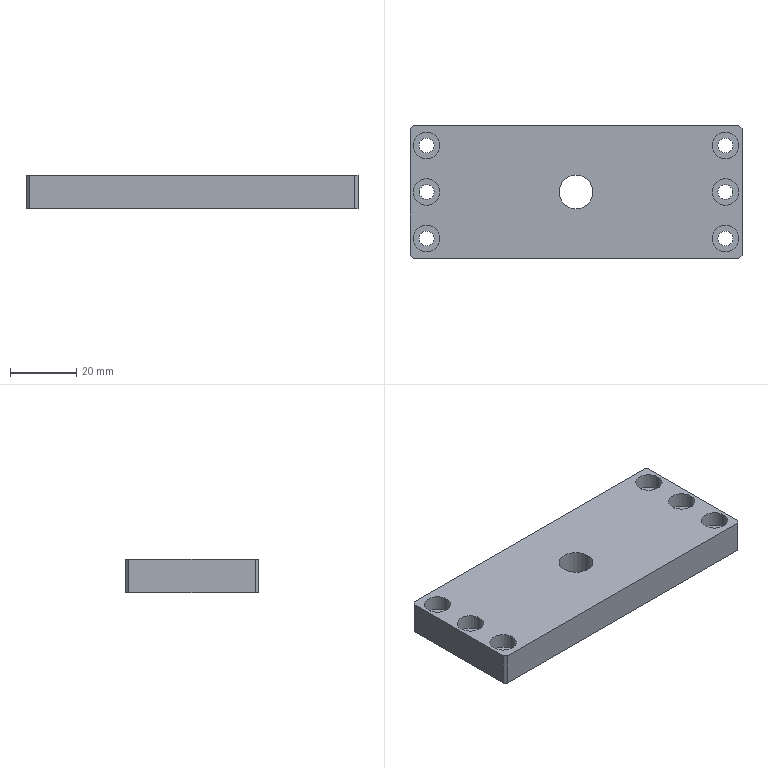Part | STEP file | MYT-A01-P12 | 1 solid | 42 faces | box 100 x 40 x 10 mm | volume 37260 mm3 | cylinder 26 | plane 16 | commonest cylinder face diameters 4.5 x12 8 x12 10.2 x2
STEP:
#1=CARTESIAN_POINT('',(-5.1,0.,0.));
#2=VERTEX_POINT('',#1);
#3=CARTESIAN_POINT('',(5.1,0.,0.));
#4=VERTEX_POINT('',#3);
#5=CARTESIAN_POINT('',(0.,0.,0.));
#6=DIRECTION('',(0.,0.,1.));
#7=DIRECTION('',(1.,0.,0.));
#8=AXIS2_PLACEMENT_3D('',#5,#6,#7);
#9=CIRCLE('',#8,5.1);
#10=EDGE_CURVE('',#2,#4,#9,.T.);
#11=ORIENTED_EDGE('',*,*,#10,.F.);
#12=CARTESIAN_POINT('',(-5.1,0.,10.));
#13=VERTEX_POINT('',#12);
#14=CARTESIAN_POINT('',(-5.1,0.,10.));
#15=DIRECTION('',(0.,0.,1.));
#16=VECTOR('',#15,1000.);
#17=LINE('',#14,#16);
#18=EDGE_CURVE('',#2,#13,#17,.T.);
#19=ORIENTED_EDGE('',*,*,#18,.T.);
#20=CARTESIAN_POINT('',(5.1,0.,10.));
#21=VERTEX_POINT('',#20);
#22=CARTESIAN_POINT('',(0.,0.,10.));
#23=DIRECTION('',(0.,0.,1.));
#24=DIRECTION('',(1.,0.,0.));
#25=AXIS2_PLACEMENT_3D('',#22,#23,#24);
#26=CIRCLE('',#25,5.1);
#27=EDGE_CURVE('',#13,#21,#26,.T.);
#28=ORIENTED_EDGE('',*,*,#27,.T.);
#29=CARTESIAN_POINT('',(5.1,0.,10.));
#30=DIRECTION('',(0.,0.,1.));
#31=VECTOR('',#30,1000.);
#32=LINE('',#29,#31);
#33=EDGE_CURVE('',#4,#21,#32,.T.);
#34=ORIENTED_EDGE('',*,*,#33,.F.);
#35=EDGE_LOOP('',(#11,#19,#28,#34));
#36=FACE_OUTER_BOUND('',#35,.T.);
#37=CARTESIAN_POINT('',(0.,0.,10.));
#38=DIRECTION('',(0.,0.,1.));
#39=DIRECTION('',(1.,0.,0.));
#40=AXIS2_PLACEMENT_3D('',#37,#38,#39);
#41=CYLINDRICAL_SURFACE('',#40,5.1);
#42=ADVANCED_FACE('',(#36),#41,.F.);
#43=CARTESIAN_POINT('',(-49.,14.,5.4));
#44=VERTEX_POINT('',#43);
#45=CARTESIAN_POINT('',(-41.,14.,5.4));
#46=VERTEX_POINT('',#45);
#47=CARTESIAN_POINT('',(-45.,14.,5.4));
#48=DIRECTION('',(0.,0.,1.));
#49=DIRECTION('',(1.,0.,0.));
#50=AXIS2_PLACEMENT_3D('',#47,#48,#49);
#51=CIRCLE('',#50,4.);
#52=EDGE_CURVE('',#44,#46,#51,.T.);
#53=ORIENTED_EDGE('',*,*,#52,.F.);
#54=CARTESIAN_POINT('',(-49.,14.,10.));
#55=VERTEX_POINT('',#54);
#56=CARTESIAN_POINT('',(-49.,14.,10.));
#57=DIRECTION('',(0.,0.,1.));
#58=VECTOR('',#57,1000.);
#59=LINE('',#56,#58);
#60=EDGE_CURVE('',#44,#55,#59,.T.);
#61=ORIENTED_EDGE('',*,*,#60,.T.);
#62=CARTESIAN_POINT('',(-41.,14.,10.));
#63=VERTEX_POINT('',#62);
#64=CARTESIAN_POINT('',(-45.,14.,10.));
#65=DIRECTION('',(0.,0.,1.));
#66=DIRECTION('',(1.,0.,0.));
#67=AXIS2_PLACEMENT_3D('',#64,#65,#66);
#68=CIRCLE('',#67,4.);
#69=EDGE_CURVE('',#55,#63,#68,.T.);
#70=ORIENTED_EDGE('',*,*,#69,.T.);
#71=CARTESIAN_POINT('',(-41.,14.,10.));
#72=DIRECTION('',(0.,0.,1.));
#73=VECTOR('',#72,1000.);
#74=LINE('',#71,#73);
#75=EDGE_CURVE('',#46,#63,#74,.T.);
#76=ORIENTED_EDGE('',*,*,#75,.F.);
#77=EDGE_LOOP('',(#53,#61,#70,#76));
#78=FACE_OUTER_BOUND('',#77,.T.);
#79=CARTESIAN_POINT('',(-45.,14.,10.));
#80=DIRECTION('',(0.,0.,1.));
#81=DIRECTION('',(1.,0.,0.));
#82=AXIS2_PLACEMENT_3D('',#79,#80,#81);
#83=CYLINDRICAL_SURFACE('',#82,4.);
#84=ADVANCED_FACE('',(#78),#83,.F.);
#85=CARTESIAN_POINT('',(-42.75,14.,0.));
#86=VERTEX_POINT('',#85);
#87=CARTESIAN_POINT('',(-47.25,14.,0.));
#88=VERTEX_POINT('',#87);
#89=CARTESIAN_POINT('',(-45.,14.,0.));
#90=DIRECTION('',(0.,0.,-1.));
#91=DIRECTION('',(-1.,0.,0.));
#92=AXIS2_PLACEMENT_3D('',#89,#90,#91);
#93=CIRCLE('',#92,2.25);
#94=EDGE_CURVE('',#86,#88,#93,.T.);
#95=ORIENTED_EDGE('',*,*,#94,.T.);
#96=CARTESIAN_POINT('',(-47.25,14.,5.4));
#97=VERTEX_POINT('',#96);
#98=CARTESIAN_POINT('',(-47.25,14.,10.));
#99=DIRECTION('',(0.,0.,1.));
#100=VECTOR('',#99,1000.);
#101=LINE('',#98,#100);
#102=EDGE_CURVE('',#88,#97,#101,.T.);
#103=ORIENTED_EDGE('',*,*,#102,.T.);
#104=CARTESIAN_POINT('',(-42.75,14.,5.4));
#105=VERTEX_POINT('',#104);
#106=CARTESIAN_POINT('',(-45.,14.,5.4));
#107=DIRECTION('',(0.,0.,1.));
#108=DIRECTION('',(1.,0.,0.));
#109=AXIS2_PLACEMENT_3D('',#106,#107,#108);
#110=CIRCLE('',#109,2.25);
#111=EDGE_CURVE('',#97,#105,#110,.T.);
#112=ORIENTED_EDGE('',*,*,#111,.T.);
#113=CARTESIAN_POINT('',(-42.75,14.,10.));
#114=DIRECTION('',(0.,0.,1.));
#115=VECTOR('',#114,1000.);
#116=LINE('',#113,#115);
#117=EDGE_CURVE('',#86,#105,#116,.T.);
#118=ORIENTED_EDGE('',*,*,#117,.F.);
#119=EDGE_LOOP('',(#95,#103,#112,#118));
#120=FACE_OUTER_BOUND('',#119,.T.);
#121=CARTESIAN_POINT('',(-45.,14.,10.));
#122=DIRECTION('',(0.,0.,1.));
#123=DIRECTION('',(1.,0.,0.));
#124=AXIS2_PLACEMENT_3D('',#121,#122,#123);
#125=CYLINDRICAL_SURFACE('',#124,2.25);
#126=ADVANCED_FACE('',(#120),#125,.F.);
#127=CARTESIAN_POINT('',(-49.,0.,5.4));
#128=VERTEX_POINT('',#127);
#129=CARTESIAN_POINT('',(-41.,0.,5.4));
#130=VERTEX_POINT('',#129);
#131=CARTESIAN_POINT('',(-45.,0.,5.4));
#132=DIRECTION('',(0.,0.,1.));
#133=DIRECTION('',(1.,0.,0.));
#134=AXIS2_PLACEMENT_3D('',#131,#132,#133);
#135=CIRCLE('',#134,4.);
#136=EDGE_CURVE('',#128,#130,#135,.T.);
#137=ORIENTED_EDGE('',*,*,#136,.F.);
#138=CARTESIAN_POINT('',(-49.,0.,10.));
#139=VERTEX_POINT('',#138);
#140=CARTESIAN_POINT('',(-49.,0.,10.));
#141=DIRECTION('',(0.,0.,1.));
#142=VECTOR('',#141,1000.);
#143=LINE('',#140,#142);
#144=EDGE_CURVE('',#128,#139,#143,.T.);
#145=ORIENTED_EDGE('',*,*,#144,.T.);
#146=CARTESIAN_POINT('',(-41.,0.,10.));
#147=VERTEX_POINT('',#146);
#148=CARTESIAN_POINT('',(-45.,0.,10.));
#149=DIRECTION('',(0.,0.,1.));
#150=DIRECTION('',(1.,0.,0.));
#151=AXIS2_PLACEMENT_3D('',#148,#149,#150);
#152=CIRCLE('',#151,4.);
#153=EDGE_CURVE('',#139,#147,#152,.T.);
#154=ORIENTED_EDGE('',*,*,#153,.T.);
#155=CARTESIAN_POINT('',(-41.,0.,10.));
#156=DIRECTION('',(0.,0.,1.));
#157=VECTOR('',#156,1000.);
#158=LINE('',#155,#157);
#159=EDGE_CURVE('',#130,#147,#158,.T.);
#160=ORIENTED_EDGE('',*,*,#159,.F.);
#161=EDGE_LOOP('',(#137,#145,#154,#160));
#162=FACE_OUTER_BOUND('',#161,.T.);
#163=CARTESIAN_POINT('',(-45.,0.,10.));
#164=DIRECTION('',(0.,0.,1.));
#165=DIRECTION('',(1.,0.,0.));
#166=AXIS2_PLACEMENT_3D('',#163,#164,#165);
#167=CYLINDRICAL_SURFACE('',#166,4.);
#168=ADVANCED_FACE('',(#162),#167,.F.);
#169=CARTESIAN_POINT('',(-42.75,0.,0.));
#170=VERTEX_POINT('',#169);
#171=CARTESIAN_POINT('',(-47.25,0.,0.));
#172=VERTEX_POINT('',#171);
#173=CARTESIAN_POINT('',(-45.,0.,0.));
#174=DIRECTION('',(0.,0.,-1.));
#175=DIRECTION('',(-1.,0.,0.));
#176=AXIS2_PLACEMENT_3D('',#173,#174,#175);
#177=CIRCLE('',#176,2.25);
#178=EDGE_CURVE('',#170,#172,#177,.T.);
#179=ORIENTED_EDGE('',*,*,#178,.T.);
#180=CARTESIAN_POINT('',(-47.25,0.,5.4));
#181=VERTEX_POINT('',#180);
#182=CARTESIAN_POINT('',(-47.25,0.,10.));
#183=DIRECTION('',(0.,0.,1.));
#184=VECTOR('',#183,1000.);
#185=LINE('',#182,#184);
#186=EDGE_CURVE('',#172,#181,#185,.T.);
#187=ORIENTED_EDGE('',*,*,#186,.T.);
#188=CARTESIAN_POINT('',(-42.75,0.,5.4));
#189=VERTEX_POINT('',#188);
#190=CARTESIAN_POINT('',(-45.,0.,5.4));
#191=DIRECTION('',(0.,0.,1.));
#192=DIRECTION('',(1.,0.,0.));
#193=AXIS2_PLACEMENT_3D('',#190,#191,#192);
#194=CIRCLE('',#193,2.25);
#195=EDGE_CURVE('',#181,#189,#194,.T.);
#196=ORIENTED_EDGE('',*,*,#195,.T.);
#197=CARTESIAN_POINT('',(-42.75,0.,10.));
#198=DIRECTION('',(0.,0.,1.));
#199=VECTOR('',#198,1000.);
#200=LINE('',#197,#199);
#201=EDGE_CURVE('',#170,#189,#200,.T.);
#202=ORIENTED_EDGE('',*,*,#201,.F.);
#203=EDGE_LOOP('',(#179,#187,#196,#202));
#204=FACE_OUTER_BOUND('',#203,.T.);
#205=CARTESIAN_POINT('',(-45.,0.,10.));
#206=DIRECTION('',(0.,0.,1.));
#207=DIRECTION('',(1.,0.,0.));
#208=AXIS2_PLACEMENT_3D('',#205,#206,#207);
#209=CYLINDRICAL_SURFACE('',#208,2.25);
#210=ADVANCED_FACE('',(#204),#209,.F.);
#211=CARTESIAN_POINT('',(-49.,-14.,5.4));
#212=VERTEX_POINT('',#211);
#213=CARTESIAN_POINT('',(-41.,-14.,5.4));
#214=VERTEX_POINT('',#213);
#215=CARTESIAN_POINT('',(-45.,-14.,5.4));
#216=DIRECTION('',(0.,0.,1.));
#217=DIRECTION('',(1.,0.,0.));
#218=AXIS2_PLACEMENT_3D('',#215,#216,#217);
#219=CIRCLE('',#218,4.);
#220=EDGE_CURVE('',#212,#214,#219,.T.);
#221=ORIENTED_EDGE('',*,*,#220,.F.);
#222=CARTESIAN_POINT('',(-49.,-14.,10.));
#223=VERTEX_POINT('',#222);
#224=CARTESIAN_POINT('',(-49.,-14.,10.));
#225=DIRECTION('',(0.,0.,1.));
#226=VECTOR('',#225,1000.);
#227=LINE('',#224,#226);
#228=EDGE_CURVE('',#212,#223,#227,.T.);
#229=ORIENTED_EDGE('',*,*,#228,.T.);
#230=CARTESIAN_POINT('',(-41.,-14.,10.));
#231=VERTEX_POINT('',#230);
#232=CARTESIAN_POINT('',(-45.,-14.,10.));
#233=DIRECTION('',(0.,0.,1.));
#234=DIRECTION('',(1.,0.,0.));
#235=AXIS2_PLACEMENT_3D('',#232,#233,#234);
#236=CIRCLE('',#235,4.);
#237=EDGE_CURVE('',#223,#231,#236,.T.);
#238=ORIENTED_EDGE('',*,*,#237,.T.);
#239=CARTESIAN_POINT('',(-41.,-14.,10.));
#240=DIRECTION('',(0.,0.,1.));
#241=VECTOR('',#240,1000.);
#242=LINE('',#239,#241);
#243=EDGE_CURVE('',#214,#231,#242,.T.);
#244=ORIENTED_EDGE('',*,*,#243,.F.);
#245=EDGE_LOOP('',(#221,#229,#238,#244));
#246=FACE_OUTER_BOUND('',#245,.T.);
#247=CARTESIAN_POINT('',(-45.,-14.,10.));
#248=DIRECTION('',(0.,0.,1.));
#249=DIRECTION('',(1.,0.,0.));
#250=AXIS2_PLACEMENT_3D('',#247,#248,#249);
#251=CYLINDRICAL_SURFACE('',#250,4.);
#252=ADVANCED_FACE('',(#246),#251,.F.);
#253=CARTESIAN_POINT('',(-42.75,-14.,0.));
#254=VERTEX_POINT('',#253);
#255=CARTESIAN_POINT('',(-47.25,-14.,0.));
#256=VERTEX_POINT('',#255);
#257=CARTESIAN_POINT('',(-45.,-14.,0.));
#258=DIRECTION('',(0.,0.,-1.));
#259=DIRECTION('',(-1.,0.,0.));
#260=AXIS2_PLACEMENT_3D('',#257,#258,#259);
#261=CIRCLE('',#260,2.25);
#262=EDGE_CURVE('',#254,#256,#261,.T.);
#263=ORIENTED_EDGE('',*,*,#262,.T.);
#264=CARTESIAN_POINT('',(-47.25,-14.,5.4));
#265=VERTEX_POINT('',#264);
#266=CARTESIAN_POINT('',(-47.25,-14.,10.));
#267=DIRECTION('',(0.,0.,1.));
#268=VECTOR('',#267,1000.);
#269=LINE('',#266,#268);
#270=EDGE_CURVE('',#256,#265,#269,.T.);
#271=ORIENTED_EDGE('',*,*,#270,.T.);
#272=CARTESIAN_POINT('',(-42.75,-14.,5.4));
#273=VERTEX_POINT('',#272);
#274=CARTESIAN_POINT('',(-45.,-14.,5.4));
#275=DIRECTION('',(0.,0.,1.));
#276=DIRECTION('',(1.,0.,0.));
#277=AXIS2_PLACEMENT_3D('',#274,#275,#276);
#278=CIRCLE('',#277,2.25);
#279=EDGE_CURVE('',#265,#273,#278,.T.);
#280=ORIENTED_EDGE('',*,*,#279,.T.);
#281=CARTESIAN_POINT('',(-42.75,-14.,10.));
#282=DIRECTION('',(0.,0.,1.));
#283=VECTOR('',#282,1000.);
#284=LINE('',#281,#283);
#285=EDGE_CURVE('',#254,#273,#284,.T.);
#286=ORIENTED_EDGE('',*,*,#285,.F.);
#287=EDGE_LOOP('',(#263,#271,#280,#286));
#288=FACE_OUTER_BOUND('',#287,.T.);
#289=CARTESIAN_POINT('',(-45.,-14.,10.));
#290=DIRECTION('',(0.,0.,1.));
#291=DIRECTION('',(1.,0.,0.));
#292=AXIS2_PLACEMENT_3D('',#289,#290,#291);
#293=CYLINDRICAL_SURFACE('',#292,2.25);
#294=ADVANCED_FACE('',(#288),#293,.F.);
#295=CARTESIAN_POINT('',(41.,-14.,5.4));
#296=VERTEX_POINT('',#295);
#297=CARTESIAN_POINT('',(49.,-14.,5.4));
#298=VERTEX_POINT('',#297);
#299=CARTESIAN_POINT('',(45.,-14.,5.4));
#300=DIRECTION('',(0.,0.,1.));
#301=DIRECTION('',(1.,0.,0.));
#302=AXIS2_PLACEMENT_3D('',#299,#300,#301);
#303=CIRCLE('',#302,4.);
#304=EDGE_CURVE('',#296,#298,#303,.T.);
#305=ORIENTED_EDGE('',*,*,#304,.F.);
#306=CARTESIAN_POINT('',(41.,-14.,10.));
#307=VERTEX_POINT('',#306);
#308=CARTESIAN_POINT('',(41.,-14.,10.));
#309=DIRECTION('',(0.,0.,1.));
#310=VECTOR('',#309,1000.);
#311=LINE('',#308,#310);
#312=EDGE_CURVE('',#296,#307,#311,.T.);
#313=ORIENTED_EDGE('',*,*,#312,.T.);
#314=CARTESIAN_POINT('',(49.,-14.,10.));
#315=VERTEX_POINT('',#314);
#316=CARTESIAN_POINT('',(45.,-14.,10.));
#317=DIRECTION('',(0.,0.,1.));
#318=DIRECTION('',(1.,0.,0.));
#319=AXIS2_PLACEMENT_3D('',#316,#317,#318);
#320=CIRCLE('',#319,4.);
#321=EDGE_CURVE('',#307,#315,#320,.T.);
#322=ORIENTED_EDGE('',*,*,#321,.T.);
#323=CARTESIAN_POINT('',(49.,-14.,10.));
#324=DIRECTION('',(0.,0.,1.));
#325=VECTOR('',#324,1000.);
#326=LINE('',#323,#325);
#327=EDGE_CURVE('',#298,#315,#326,.T.);
#328=ORIENTED_EDGE('',*,*,#327,.F.);
#329=EDGE_LOOP('',(#305,#313,#322,#328));
#330=FACE_OUTER_BOUND('',#329,.T.);
#331=CARTESIAN_POINT('',(45.,-14.,10.));
#332=DIRECTION('',(0.,0.,1.));
#333=DIRECTION('',(1.,0.,0.));
#334=AXIS2_PLACEMENT_3D('',#331,#332,#333);
#335=CYLINDRICAL_SURFACE('',#334,4.);
#336=ADVANCED_FACE('',(#330),#335,.F.);
#337=CARTESIAN_POINT('',(47.25,-14.,0.));
#338=VERTEX_POINT('',#337);
#339=CARTESIAN_POINT('',(42.75,-14.,0.));
#340=VERTEX_POINT('',#339);
#341=CARTESIAN_POINT('',(45.,-14.,0.));
#342=DIRECTION('',(0.,0.,-1.));
#343=DIRECTION('',(-1.,0.,0.));
#344=AXIS2_PLACEMENT_3D('',#341,#342,#343);
#345=CIRCLE('',#344,2.25);
#346=EDGE_CURVE('',#338,#340,#345,.T.);
#347=ORIENTED_EDGE('',*,*,#346,.T.);
#348=CARTESIAN_POINT('',(42.75,-14.,5.4));
#349=VERTEX_POINT('',#348);
#350=CARTESIAN_POINT('',(42.75,-14.,10.));
#351=DIRECTION('',(0.,0.,1.));
#352=VECTOR('',#351,1000.);
#353=LINE('',#350,#352);
#354=EDGE_CURVE('',#340,#349,#353,.T.);
#355=ORIENTED_EDGE('',*,*,#354,.T.);
#356=CARTESIAN_POINT('',(47.25,-14.,5.4));
#357=VERTEX_POINT('',#356);
#358=CARTESIAN_POINT('',(45.,-14.,5.4));
#359=DIRECTION('',(0.,0.,1.));
#360=DIRECTION('',(1.,0.,0.));
#361=AXIS2_PLACEMENT_3D('',#358,#359,#360);
#362=CIRCLE('',#361,2.25);
#363=EDGE_CURVE('',#349,#357,#362,.T.);
#364=ORIENTED_EDGE('',*,*,#363,.T.);
#365=CARTESIAN_POINT('',(47.25,-14.,10.));
#366=DIRECTION('',(0.,0.,1.));
#367=VECTOR('',#366,1000.);
#368=LINE('',#365,#367);
#369=EDGE_CURVE('',#338,#357,#368,.T.);
#370=ORIENTED_EDGE('',*,*,#369,.F.);
#371=EDGE_LOOP('',(#347,#355,#364,#370));
#372=FACE_OUTER_BOUND('',#371,.T.);
#373=CARTESIAN_POINT('',(45.,-14.,10.));
#374=DIRECTION('',(0.,0.,1.));
#375=DIRECTION('',(1.,0.,0.));
#376=AXIS2_PLACEMENT_3D('',#373,#374,#375);
#377=CYLINDRICAL_SURFACE('',#376,2.25);
#378=ADVANCED_FACE('',(#372),#377,.F.);
#379=CARTESIAN_POINT('',(41.,0.,5.4));
#380=VERTEX_POINT('',#379);
#381=CARTESIAN_POINT('',(49.,0.,5.4));
#382=VERTEX_POINT('',#381);
#383=CARTESIAN_POINT('',(45.,0.,5.4));
#384=DIRECTION('',(0.,0.,1.));
#385=DIRECTION('',(1.,0.,0.));
#386=AXIS2_PLACEMENT_3D('',#383,#384,#385);
#387=CIRCLE('',#386,4.);
#388=EDGE_CURVE('',#380,#382,#387,.T.);
#389=ORIENTED_EDGE('',*,*,#388,.F.);
#390=CARTESIAN_POINT('',(41.,0.,10.));
#391=VERTEX_POINT('',#390);
#392=CARTESIAN_POINT('',(41.,0.,10.));
#393=DIRECTION('',(0.,0.,1.));
#394=VECTOR('',#393,1000.);
#395=LINE('',#392,#394);
#396=EDGE_CURVE('',#380,#391,#395,.T.);
#397=ORIENTED_EDGE('',*,*,#396,.T.);
#398=CARTESIAN_POINT('',(49.,0.,10.));
#399=VERTEX_POINT('',#398);
#400=CARTESIAN_POINT('',(45.,0.,10.));
#401=DIRECTION('',(0.,0.,1.));
#402=DIRECTION('',(1.,0.,0.));
#403=AXIS2_PLACEMENT_3D('',#400,#401,#402);
#404=CIRCLE('',#403,4.);
#405=EDGE_CURVE('',#391,#399,#404,.T.);
#406=ORIENTED_EDGE('',*,*,#405,.T.);
#407=CARTESIAN_POINT('',(49.,0.,10.));
#408=DIRECTION('',(0.,0.,1.));
#409=VECTOR('',#408,1000.);
#410=LINE('',#407,#409);
#411=EDGE_CURVE('',#382,#399,#410,.T.);
#412=ORIENTED_EDGE('',*,*,#411,.F.);
#413=EDGE_LOOP('',(#389,#397,#406,#412));
#414=FACE_OUTER_BOUND('',#413,.T.);
#415=CARTESIAN_POINT('',(45.,0.,10.));
#416=DIRECTION('',(0.,0.,1.));
#417=DIRECTION('',(1.,0.,0.));
#418=AXIS2_PLACEMENT_3D('',#415,#416,#417);
#419=CYLINDRICAL_SURFACE('',#418,4.);
#420=ADVANCED_FACE('',(#414),#419,.F.);
#421=CARTESIAN_POINT('',(47.25,0.,0.));
#422=VERTEX_POINT('',#421);
#423=CARTESIAN_POINT('',(42.75,0.,0.));
#424=VERTEX_POINT('',#423);
#425=CARTESIAN_POINT('',(45.,0.,0.));
#426=DIRECTION('',(0.,0.,-1.));
#427=DIRECTION('',(-1.,0.,0.));
#428=AXIS2_PLACEMENT_3D('',#425,#426,#427);
#429=CIRCLE('',#428,2.25);
#430=EDGE_CURVE('',#422,#424,#429,.T.);
#431=ORIENTED_EDGE('',*,*,#430,.T.);
#432=CARTESIAN_POINT('',(42.75,0.,5.4));
#433=VERTEX_POINT('',#432);
#434=CARTESIAN_POINT('',(42.75,0.,10.));
#435=DIRECTION('',(0.,0.,1.));
#436=VECTOR('',#435,1000.);
#437=LINE('',#434,#436);
#438=EDGE_CURVE('',#424,#433,#437,.T.);
#439=ORIENTED_EDGE('',*,*,#438,.T.);
#440=CARTESIAN_POINT('',(47.25,0.,5.4));
#441=VERTEX_POINT('',#440);
#442=CARTESIAN_POINT('',(45.,0.,5.4));
#443=DIRECTION('',(0.,0.,1.));
#444=DIRECTION('',(1.,0.,0.));
#445=AXIS2_PLACEMENT_3D('',#442,#443,#444);
#446=CIRCLE('',#445,2.25);
#447=EDGE_CURVE('',#433,#441,#446,.T.);
#448=ORIENTED_EDGE('',*,*,#447,.T.);
#449=CARTESIAN_POINT('',(47.25,0.,10.));
#450=DIRECTION('',(0.,0.,1.));
#451=VECTOR('',#450,1000.);
#452=LINE('',#449,#451);
#453=EDGE_CURVE('',#422,#441,#452,.T.);
#454=ORIENTED_EDGE('',*,*,#453,.F.);
#455=EDGE_LOOP('',(#431,#439,#448,#454));
#456=FACE_OUTER_BOUND('',#455,.T.);
#457=CARTESIAN_POINT('',(45.,0.,10.));
#458=DIRECTION('',(0.,0.,1.));
#459=DIRECTION('',(1.,0.,0.));
#460=AXIS2_PLACEMENT_3D('',#457,#458,#459);
#461=CYLINDRICAL_SURFACE('',#460,2.25);
#462=ADVANCED_FACE('',(#456),#461,.F.);
#463=CARTESIAN_POINT('',(41.,14.,5.4));
#464=VERTEX_POINT('',#463);
#465=CARTESIAN_POINT('',(49.,14.,5.4));
#466=VERTEX_POINT('',#465);
#467=CARTESIAN_POINT('',(45.,14.,5.4));
#468=DIRECTION('',(0.,0.,1.));
#469=DIRECTION('',(1.,0.,0.));
#470=AXIS2_PLACEMENT_3D('',#467,#468,#469);
#471=CIRCLE('',#470,4.);
#472=EDGE_CURVE('',#464,#466,#471,.T.);
#473=ORIENTED_EDGE('',*,*,#472,.F.);
#474=CARTESIAN_POINT('',(41.,14.,10.));
#475=VERTEX_POINT('',#474);
#476=CARTESIAN_POINT('',(41.,14.,10.));
#477=DIRECTION('',(0.,0.,1.));
#478=VECTOR('',#477,1000.);
#479=LINE('',#476,#478);
#480=EDGE_CURVE('',#464,#475,#479,.T.);
#481=ORIENTED_EDGE('',*,*,#480,.T.);
#482=CARTESIAN_POINT('',(49.,14.,10.));
#483=VERTEX_POINT('',#482);
#484=CARTESIAN_POINT('',(45.,14.,10.));
#485=DIRECTION('',(0.,0.,1.));
#486=DIRECTION('',(1.,0.,0.));
#487=AXIS2_PLACEMENT_3D('',#484,#485,#486);
#488=CIRCLE('',#487,4.);
#489=EDGE_CURVE('',#475,#483,#488,.T.);
#490=ORIENTED_EDGE('',*,*,#489,.T.);
#491=CARTESIAN_POINT('',(49.,14.,10.));
#492=DIRECTION('',(0.,0.,1.));
#493=VECTOR('',#492,1000.);
#494=LINE('',#491,#493);
#495=EDGE_CURVE('',#466,#483,#494,.T.);
#496=ORIENTED_EDGE('',*,*,#495,.F.);
#497=EDGE_LOOP('',(#473,#481,#490,#496));
#498=FACE_OUTER_BOUND('',#497,.T.);
#499=CARTESIAN_POINT('',(45.,14.,10.));
#500=DIRECTION('',(0.,0.,1.));
#501=DIRECTION('',(1.,0.,0.));
#502=AXIS2_PLACEMENT_3D('',#499,#500,#501);
#503=CYLINDRICAL_SURFACE('',#502,4.);
#504=ADVANCED_FACE('',(#498),#503,.F.);
#505=CARTESIAN_POINT('',(47.25,14.,0.));
#506=VERTEX_POINT('',#505);
#507=CARTESIAN_POINT('',(42.75,14.,0.));
#508=VERTEX_POINT('',#507);
#509=CARTESIAN_POINT('',(45.,14.,0.));
#510=DIRECTION('',(0.,0.,-1.));
#511=DIRECTION('',(-1.,0.,0.));
#512=AXIS2_PLACEMENT_3D('',#509,#510,#511);
#513=CIRCLE('',#512,2.25);
#514=EDGE_CURVE('',#506,#508,#513,.T.);
#515=ORIENTED_EDGE('',*,*,#514,.T.);
#516=CARTESIAN_POINT('',(42.75,14.,5.4));
#517=VERTEX_POINT('',#516);
#518=CARTESIAN_POINT('',(42.75,14.,10.));
#519=DIRECTION('',(0.,0.,1.));
#520=VECTOR('',#519,1000.);
#521=LINE('',#518,#520);
#522=EDGE_CURVE('',#508,#517,#521,.T.);
#523=ORIENTED_EDGE('',*,*,#522,.T.);
#524=CARTESIAN_POINT('',(47.25,14.,5.4));
#525=VERTEX_POINT('',#524);
#526=CARTESIAN_POINT('',(45.,14.,5.4));
#527=DIRECTION('',(0.,0.,1.));
#528=DIRECTION('',(1.,0.,0.));
#529=AXIS2_PLACEMENT_3D('',#526,#527,#528);
#530=CIRCLE('',#529,2.25);
#531=EDGE_CURVE('',#517,#525,#530,.T.);
#532=ORIENTED_EDGE('',*,*,#531,.T.);
#533=CARTESIAN_POINT('',(47.25,14.,10.));
#534=DIRECTION('',(0.,0.,1.));
#535=VECTOR('',#534,1000.);
#536=LINE('',#533,#535);
#537=EDGE_CURVE('',#506,#525,#536,.T.);
#538=ORIENTED_EDGE('',*,*,#537,.F.);
#539=EDGE_LOOP('',(#515,#523,#532,#538));
#540=FACE_OUTER_BOUND('',#539,.T.);
#541=CARTESIAN_POINT('',(45.,14.,10.));
#542=DIRECTION('',(0.,0.,1.));
#543=DIRECTION('',(1.,0.,0.));
#544=AXIS2_PLACEMENT_3D('',#541,#542,#543);
#545=CYLINDRICAL_SURFACE('',#544,2.25);
#546=ADVANCED_FACE('',(#540),#545,.F.);
#547=CARTESIAN_POINT('',(50.,-19.,10.));
#548=VERTEX_POINT('',#547);
#549=CARTESIAN_POINT('',(50.,19.,10.));
#550=VERTEX_POINT('',#549);
#551=CARTESIAN_POINT('',(50.,-20.,10.));
#552=DIRECTION('',(0.,1.,0.));
#553=VECTOR('',#552,1000.);
#554=LINE('',#551,#553);
#555=EDGE_CURVE('',#548,#550,#554,.T.);
#556=ORIENTED_EDGE('',*,*,#555,.F.);
#557=CARTESIAN_POINT('',(50.,-19.,0.));
#558=VERTEX_POINT('',#557);
#559=CARTESIAN_POINT('',(50.,-19.,10.));
#560=DIRECTION('',(0.,0.,-1.));
#561=VECTOR('',#560,1000.);
#562=LINE('',#559,#561);
#563=EDGE_CURVE('',#548,#558,#562,.T.);
#564=ORIENTED_EDGE('',*,*,#563,.T.);
#565=CARTESIAN_POINT('',(50.,19.,0.));
#566=VERTEX_POINT('',#565);
#567=CARTESIAN_POINT('',(50.,-20.,0.));
#568=DIRECTION('',(0.,1.,0.));
#569=VECTOR('',#568,1000.);
#570=LINE('',#567,#569);
#571=EDGE_CURVE('',#558,#566,#570,.T.);
#572=ORIENTED_EDGE('',*,*,#571,.T.);
#573=CARTESIAN_POINT('',(50.,19.,10.));
#574=DIRECTION('',(0.,0.,1.));
#575=VECTOR('',#574,1000.);
#576=LINE('',#573,#575);
#577=EDGE_CURVE('',#566,#550,#576,.T.);
#578=ORIENTED_EDGE('',*,*,#577,.T.);
#579=EDGE_LOOP('',(#556,#564,#572,#578));
#580=FACE_OUTER_BOUND('',#579,.T.);
#581=CARTESIAN_POINT('',(50.,-20.,10.));
#582=DIRECTION('',(-1.,0.,0.));
#583=DIRECTION('',(0.,0.,1.));
#584=AXIS2_PLACEMENT_3D('',#581,#582,#583);
#585=PLANE('',#584);
#586=ADVANCED_FACE('',(#580),#585,.F.);
#587=CARTESIAN_POINT('',(49.,20.,10.));
#588=VERTEX_POINT('',#587);
#589=CARTESIAN_POINT('',(-49.,20.,10.));
#590=VERTEX_POINT('',#589);
#591=CARTESIAN_POINT('',(-50.,20.,10.));
#592=DIRECTION('',(-1.,0.,0.));
#593=VECTOR('',#592,1000.);
#594=LINE('',#591,#593);
#595=EDGE_CURVE('',#588,#590,#594,.T.);
#596=ORIENTED_EDGE('',*,*,#595,.F.);
#597=CARTESIAN_POINT('',(49.,20.,0.));
#598=VERTEX_POINT('',#597);
#599=CARTESIAN_POINT('',(49.,20.,10.));
#600=DIRECTION('',(0.,0.,-1.));
#601=VECTOR('',#600,1000.);
#602=LINE('',#599,#601);
#603=EDGE_CURVE('',#588,#598,#602,.T.);
#604=ORIENTED_EDGE('',*,*,#603,.T.);
#605=CARTESIAN_POINT('',(-49.,20.,0.));
#606=VERTEX_POINT('',#605);
#607=CARTESIAN_POINT('',(-50.,20.,0.));
#608=DIRECTION('',(-1.,0.,0.));
#609=VECTOR('',#608,1000.);
#610=LINE('',#607,#609);
#611=EDGE_CURVE('',#598,#606,#610,.T.);
#612=ORIENTED_EDGE('',*,*,#611,.T.);
#613=CARTESIAN_POINT('',(-49.,20.,10.));
#614=DIRECTION('',(0.,0.,1.));
#615=VECTOR('',#614,1000.);
#616=LINE('',#613,#615);
#617=EDGE_CURVE('',#606,#590,#616,.T.);
#618=ORIENTED_EDGE('',*,*,#617,.T.);
#619=EDGE_LOOP('',(#596,#604,#612,#618));
#620=FACE_OUTER_BOUND('',#619,.T.);
#621=CARTESIAN_POINT('',(-50.,20.,10.));
#622=DIRECTION('',(0.,-1.,0.));
#623=DIRECTION('',(0.,0.,-1.));
#624=AXIS2_PLACEMENT_3D('',#621,#622,#623);
#625=PLANE('',#624);
#626=ADVANCED_FACE('',(#620),#625,.F.);
#627=CARTESIAN_POINT('',(-50.,19.,0.));
#628=VERTEX_POINT('',#627);
#629=CARTESIAN_POINT('',(-50.,-19.,0.));
#630=VERTEX_POINT('',#629);
#631=CARTESIAN_POINT('',(-50.,-20.,0.));
#632=DIRECTION('',(0.,-1.,0.));
#633=VECTOR('',#632,1000.);
#634=LINE('',#631,#633);
#635=EDGE_CURVE('',#628,#630,#634,.T.);
#636=ORIENTED_EDGE('',*,*,#635,.T.);
#637=CARTESIAN_POINT('',(-50.,-19.,10.));
#638=VERTEX_POINT('',#637);
#639=CARTESIAN_POINT('',(-50.,-19.,10.));
#640=DIRECTION('',(0.,0.,1.));
#641=VECTOR('',#640,1000.);
#642=LINE('',#639,#641);
#643=EDGE_CURVE('',#630,#638,#642,.T.);
#644=ORIENTED_EDGE('',*,*,#643,.T.);
#645=CARTESIAN_POINT('',(-50.,19.,10.));
#646=VERTEX_POINT('',#645);
#647=CARTESIAN_POINT('',(-50.,-20.,10.));
#648=DIRECTION('',(0.,-1.,0.));
#649=VECTOR('',#648,1000.);
#650=LINE('',#647,#649);
#651=EDGE_CURVE('',#646,#638,#650,.T.);
#652=ORIENTED_EDGE('',*,*,#651,.F.);
#653=CARTESIAN_POINT('',(-50.,19.,10.));
#654=DIRECTION('',(0.,0.,-1.));
#655=VECTOR('',#654,1000.);
#656=LINE('',#653,#655);
#657=EDGE_CURVE('',#646,#628,#656,.T.);
#658=ORIENTED_EDGE('',*,*,#657,.T.);
#659=EDGE_LOOP('',(#636,#644,#652,#658));
#660=FACE_OUTER_BOUND('',#659,.T.);
#661=CARTESIAN_POINT('',(-50.,-20.,10.));
#662=DIRECTION('',(1.,0.,0.));
#663=DIRECTION('',(0.,0.,-1.));
#664=AXIS2_PLACEMENT_3D('',#661,#662,#663);
#665=PLANE('',#664);
#666=ADVANCED_FACE('',(#660),#665,.F.);
#667=CARTESIAN_POINT('',(-49.,-20.,0.));
#668=VERTEX_POINT('',#667);
#669=CARTESIAN_POINT('',(49.,-20.,0.));
#670=VERTEX_POINT('',#669);
#671=CARTESIAN_POINT('',(-50.,-20.,0.));
#672=DIRECTION('',(1.,0.,0.));
#673=VECTOR('',#672,1000.);
#674=LINE('',#671,#673);
#675=EDGE_CURVE('',#668,#670,#674,.T.);
#676=ORIENTED_EDGE('',*,*,#675,.T.);
#677=CARTESIAN_POINT('',(49.,-20.,10.));
#678=VERTEX_POINT('',#677);
#679=CARTESIAN_POINT('',(49.,-20.,10.));
#680=DIRECTION('',(0.,0.,1.));
#681=VECTOR('',#680,1000.);
#682=LINE('',#679,#681);
#683=EDGE_CURVE('',#670,#678,#682,.T.);
#684=ORIENTED_EDGE('',*,*,#683,.T.);
#685=CARTESIAN_POINT('',(-49.,-20.,10.));
#686=VERTEX_POINT('',#685);
#687=CARTESIAN_POINT('',(-50.,-20.,10.));
#688=DIRECTION('',(1.,0.,0.));
#689=VECTOR('',#688,1000.);
#690=LINE('',#687,#689);
#691=EDGE_CURVE('',#686,#678,#690,.T.);
#692=ORIENTED_EDGE('',*,*,#691,.F.);
#693=CARTESIAN_POINT('',(-49.,-20.,10.));
#694=DIRECTION('',(0.,0.,-1.));
#695=VECTOR('',#694,1000.);
#696=LINE('',#693,#695);
#697=EDGE_CURVE('',#686,#668,#696,.T.);
#698=ORIENTED_EDGE('',*,*,#697,.T.);
#699=EDGE_LOOP('',(#676,#684,#692,#698));
#700=FACE_OUTER_BOUND('',#699,.T.);
#701=CARTESIAN_POINT('',(-50.,-20.,10.));
#702=DIRECTION('',(0.,1.,0.));
#703=DIRECTION('',(0.,0.,1.));
#704=AXIS2_PLACEMENT_3D('',#701,#702,#703);
#705=PLANE('',#704);
#706=ADVANCED_FACE('',(#700),#705,.F.);
#707=CARTESIAN_POINT('',(0.,0.,10.));
#708=DIRECTION('',(0.,0.,1.));
#709=DIRECTION('',(1.,0.,0.));
#710=AXIS2_PLACEMENT_3D('',#707,#708,#709);
#711=CIRCLE('',#710,5.1);
#712=EDGE_CURVE('',#21,#13,#711,.T.);
#713=ORIENTED_EDGE('',*,*,#712,.F.);
#714=ORIENTED_EDGE('',*,*,#27,.F.);
#715=EDGE_LOOP('',(#713,#714));
#716=FACE_BOUND('',#715,.T.);
#717=CARTESIAN_POINT('',(-45.,14.,10.));
#718=DIRECTION('',(0.,0.,1.));
#719=DIRECTION('',(1.,0.,0.));
#720=AXIS2_PLACEMENT_3D('',#717,#718,#719);
#721=CIRCLE('',#720,4.);
#722=EDGE_CURVE('',#63,#55,#721,.T.);
#723=ORIENTED_EDGE('',*,*,#722,.F.);
#724=ORIENTED_EDGE('',*,*,#69,.F.);
#725=EDGE_LOOP('',(#723,#724));
#726=FACE_BOUND('',#725,.T.);
#727=CARTESIAN_POINT('',(-45.,0.,10.));
#728=DIRECTION('',(0.,0.,1.));
#729=DIRECTION('',(1.,0.,0.));
#730=AXIS2_PLACEMENT_3D('',#727,#728,#729);
#731=CIRCLE('',#730,4.);
#732=EDGE_CURVE('',#147,#139,#731,.T.);
#733=ORIENTED_EDGE('',*,*,#732,.F.);
#734=ORIENTED_EDGE('',*,*,#153,.F.);
#735=EDGE_LOOP('',(#733,#734));
#736=FACE_BOUND('',#735,.T.);
#737=CARTESIAN_POINT('',(-45.,-14.,10.));
#738=DIRECTION('',(0.,0.,1.));
#739=DIRECTION('',(1.,0.,0.));
#740=AXIS2_PLACEMENT_3D('',#737,#738,#739);
#741=CIRCLE('',#740,4.);
#742=EDGE_CURVE('',#231,#223,#741,.T.);
#743=ORIENTED_EDGE('',*,*,#742,.F.);
#744=ORIENTED_EDGE('',*,*,#237,.F.);
#745=EDGE_LOOP('',(#743,#744));
#746=FACE_BOUND('',#745,.T.);
#747=CARTESIAN_POINT('',(45.,-14.,10.));
#748=DIRECTION('',(0.,0.,1.));
#749=DIRECTION('',(1.,0.,0.));
#750=AXIS2_PLACEMENT_3D('',#747,#748,#749);
#751=CIRCLE('',#750,4.);
#752=EDGE_CURVE('',#315,#307,#751,.T.);
#753=ORIENTED_EDGE('',*,*,#752,.F.);
#754=ORIENTED_EDGE('',*,*,#321,.F.);
#755=EDGE_LOOP('',(#753,#754));
#756=FACE_BOUND('',#755,.T.);
#757=CARTESIAN_POINT('',(45.,0.,10.));
#758=DIRECTION('',(0.,0.,1.));
#759=DIRECTION('',(1.,0.,0.));
#760=AXIS2_PLACEMENT_3D('',#757,#758,#759);
#761=CIRCLE('',#760,4.);
#762=EDGE_CURVE('',#399,#391,#761,.T.);
#763=ORIENTED_EDGE('',*,*,#762,.F.);
#764=ORIENTED_EDGE('',*,*,#405,.F.);
#765=EDGE_LOOP('',(#763,#764));
#766=FACE_BOUND('',#765,.T.);
#767=CARTESIAN_POINT('',(45.,14.,10.));
#768=DIRECTION('',(0.,0.,1.));
#769=DIRECTION('',(1.,0.,0.));
#770=AXIS2_PLACEMENT_3D('',#767,#768,#769);
#771=CIRCLE('',#770,4.);
#772=EDGE_CURVE('',#483,#475,#771,.T.);
#773=ORIENTED_EDGE('',*,*,#772,.F.);
#774=ORIENTED_EDGE('',*,*,#489,.F.);
#775=EDGE_LOOP('',(#773,#774));
#776=FACE_BOUND('',#775,.T.);
#777=ORIENTED_EDGE('',*,*,#691,.T.);
#778=CARTESIAN_POINT('',(50.,-19.,10.));
#779=DIRECTION('',(0.7071,0.7071,0.));
#780=VECTOR('',#779,1000.);
#781=LINE('',#778,#780);
#782=EDGE_CURVE('',#678,#548,#781,.T.);
#783=ORIENTED_EDGE('',*,*,#782,.T.);
#784=ORIENTED_EDGE('',*,*,#555,.T.);
#785=CARTESIAN_POINT('',(49.,20.,10.));
#786=DIRECTION('',(-0.7071,0.7071,0.));
#787=VECTOR('',#786,1000.);
#788=LINE('',#785,#787);
#789=EDGE_CURVE('',#550,#588,#788,.T.);
#790=ORIENTED_EDGE('',*,*,#789,.T.);
#791=ORIENTED_EDGE('',*,*,#595,.T.);
#792=CARTESIAN_POINT('',(-50.,19.,10.));
#793=DIRECTION('',(-0.7071,-0.7071,0.));
#794=VECTOR('',#793,1000.);
#795=LINE('',#792,#794);
#796=EDGE_CURVE('',#590,#646,#795,.T.);
#797=ORIENTED_EDGE('',*,*,#796,.T.);
#798=ORIENTED_EDGE('',*,*,#651,.T.);
#799=CARTESIAN_POINT('',(-49.,-20.,10.));
#800=DIRECTION('',(0.7071,-0.7071,0.));
#801=VECTOR('',#800,1000.);
#802=LINE('',#799,#801);
#803=EDGE_CURVE('',#638,#686,#802,.T.);
#804=ORIENTED_EDGE('',*,*,#803,.T.);
#805=EDGE_LOOP('',(#777,#783,#784,#790,#791,#797,#798,#804));
#806=FACE_OUTER_BOUND('',#805,.T.);
#807=CARTESIAN_POINT('',(0.,0.,10.));
#808=DIRECTION('',(0.,0.,-1.));
#809=DIRECTION('',(-1.,0.,0.));
#810=AXIS2_PLACEMENT_3D('',#807,#808,#809);
#811=PLANE('',#810);
#812=ADVANCED_FACE('',(#716,#726,#736,#746,#756,#766,#776,#806),#811,.F.);
#813=CARTESIAN_POINT('',(0.,0.,0.));
#814=DIRECTION('',(0.,0.,1.));
#815=DIRECTION('',(1.,0.,0.));
#816=AXIS2_PLACEMENT_3D('',#813,#814,#815);
#817=CIRCLE('',#816,5.1);
#818=EDGE_CURVE('',#4,#2,#817,.T.);
#819=ORIENTED_EDGE('',*,*,#818,.T.);
#820=ORIENTED_EDGE('',*,*,#10,.T.);
#821=EDGE_LOOP('',(#819,#820));
#822=FACE_BOUND('',#821,.T.);
#823=ORIENTED_EDGE('',*,*,#94,.F.);
#824=CARTESIAN_POINT('',(-45.,14.,0.));
#825=DIRECTION('',(0.,0.,-1.));
#826=DIRECTION('',(-1.,0.,0.));
#827=AXIS2_PLACEMENT_3D('',#824,#825,#826);
#828=CIRCLE('',#827,2.25);
#829=EDGE_CURVE('',#88,#86,#828,.T.);
#830=ORIENTED_EDGE('',*,*,#829,.F.);
#831=EDGE_LOOP('',(#823,#830));
#832=FACE_BOUND('',#831,.T.);
#833=ORIENTED_EDGE('',*,*,#178,.F.);
#834=CARTESIAN_POINT('',(-45.,0.,0.));
#835=DIRECTION('',(0.,0.,-1.));
#836=DIRECTION('',(-1.,0.,0.));
#837=AXIS2_PLACEMENT_3D('',#834,#835,#836);
#838=CIRCLE('',#837,2.25);
#839=EDGE_CURVE('',#172,#170,#838,.T.);
#840=ORIENTED_EDGE('',*,*,#839,.F.);
#841=EDGE_LOOP('',(#833,#840));
#842=FACE_BOUND('',#841,.T.);
#843=ORIENTED_EDGE('',*,*,#262,.F.);
#844=CARTESIAN_POINT('',(-45.,-14.,0.));
#845=DIRECTION('',(0.,0.,-1.));
#846=DIRECTION('',(-1.,0.,0.));
#847=AXIS2_PLACEMENT_3D('',#844,#845,#846);
#848=CIRCLE('',#847,2.25);
#849=EDGE_CURVE('',#256,#254,#848,.T.);
#850=ORIENTED_EDGE('',*,*,#849,.F.);
#851=EDGE_LOOP('',(#843,#850));
#852=FACE_BOUND('',#851,.T.);
#853=ORIENTED_EDGE('',*,*,#346,.F.);
#854=CARTESIAN_POINT('',(45.,-14.,0.));
#855=DIRECTION('',(0.,0.,-1.));
#856=DIRECTION('',(-1.,0.,0.));
#857=AXIS2_PLACEMENT_3D('',#854,#855,#856);
#858=CIRCLE('',#857,2.25);
#859=EDGE_CURVE('',#340,#338,#858,.T.);
#860=ORIENTED_EDGE('',*,*,#859,.F.);
#861=EDGE_LOOP('',(#853,#860));
#862=FACE_BOUND('',#861,.T.);
#863=ORIENTED_EDGE('',*,*,#430,.F.);
#864=CARTESIAN_POINT('',(45.,0.,0.));
#865=DIRECTION('',(0.,0.,-1.));
#866=DIRECTION('',(-1.,0.,0.));
#867=AXIS2_PLACEMENT_3D('',#864,#865,#866);
#868=CIRCLE('',#867,2.25);
#869=EDGE_CURVE('',#424,#422,#868,.T.);
#870=ORIENTED_EDGE('',*,*,#869,.F.);
#871=EDGE_LOOP('',(#863,#870));
#872=FACE_BOUND('',#871,.T.);
#873=ORIENTED_EDGE('',*,*,#514,.F.);
#874=CARTESIAN_POINT('',(45.,14.,0.));
#875=DIRECTION('',(0.,0.,-1.));
#876=DIRECTION('',(-1.,0.,0.));
#877=AXIS2_PLACEMENT_3D('',#874,#875,#876);
#878=CIRCLE('',#877,2.25);
#879=EDGE_CURVE('',#508,#506,#878,.T.);
#880=ORIENTED_EDGE('',*,*,#879,.F.);
#881=EDGE_LOOP('',(#873,#880));
#882=FACE_BOUND('',#881,.T.);
#883=ORIENTED_EDGE('',*,*,#571,.F.);
#884=CARTESIAN_POINT('',(34.5,-34.5,0.));
#885=DIRECTION('',(-0.7071,-0.7071,0.));
#886=VECTOR('',#885,1000.);
#887=LINE('',#884,#886);
#888=EDGE_CURVE('',#558,#670,#887,.T.);
#889=ORIENTED_EDGE('',*,*,#888,.T.);
#890=ORIENTED_EDGE('',*,*,#675,.F.);
#891=CARTESIAN_POINT('',(-34.5,-34.5,0.));
#892=DIRECTION('',(-0.7071,0.7071,0.));
#893=VECTOR('',#892,1000.);
#894=LINE('',#891,#893);
#895=EDGE_CURVE('',#668,#630,#894,.T.);
#896=ORIENTED_EDGE('',*,*,#895,.T.);
#897=ORIENTED_EDGE('',*,*,#635,.F.);
#898=CARTESIAN_POINT('',(-34.5,34.5,0.));
#899=DIRECTION('',(0.7071,0.7071,0.));
#900=VECTOR('',#899,1000.);
#901=LINE('',#898,#900);
#902=EDGE_CURVE('',#628,#606,#901,.T.);
#903=ORIENTED_EDGE('',*,*,#902,.T.);
#904=ORIENTED_EDGE('',*,*,#611,.F.);
#905=CARTESIAN_POINT('',(34.5,34.5,0.));
#906=DIRECTION('',(0.7071,-0.7071,0.));
#907=VECTOR('',#906,1000.);
#908=LINE('',#905,#907);
#909=EDGE_CURVE('',#598,#566,#908,.T.);
#910=ORIENTED_EDGE('',*,*,#909,.T.);
#911=EDGE_LOOP('',(#883,#889,#890,#896,#897,#903,#904,#910));
#912=FACE_OUTER_BOUND('',#911,.T.);
#913=CARTESIAN_POINT('',(0.,0.,0.));
#914=DIRECTION('',(0.,0.,-1.));
#915=DIRECTION('',(-1.,0.,0.));
#916=AXIS2_PLACEMENT_3D('',#913,#914,#915);
#917=PLANE('',#916);
#918=ADVANCED_FACE('',(#822,#832,#842,#852,#862,#872,#882,#912),#917,.T.);
#919=ORIENTED_EDGE('',*,*,#522,.F.);
#920=ORIENTED_EDGE('',*,*,#879,.T.);
#921=ORIENTED_EDGE('',*,*,#537,.T.);
#922=CARTESIAN_POINT('',(45.,14.,5.4));
#923=DIRECTION('',(0.,0.,1.));
#924=DIRECTION('',(1.,0.,0.));
#925=AXIS2_PLACEMENT_3D('',#922,#923,#924);
#926=CIRCLE('',#925,2.25);
#927=EDGE_CURVE('',#525,#517,#926,.T.);
#928=ORIENTED_EDGE('',*,*,#927,.T.);
#929=EDGE_LOOP('',(#919,#920,#921,#928));
#930=FACE_OUTER_BOUND('',#929,.T.);
#931=CARTESIAN_POINT('',(45.,14.,10.));
#932=DIRECTION('',(0.,0.,1.));
#933=DIRECTION('',(1.,0.,0.));
#934=AXIS2_PLACEMENT_3D('',#931,#932,#933);
#935=CYLINDRICAL_SURFACE('',#934,2.25);
#936=ADVANCED_FACE('',(#930),#935,.F.);
#937=ORIENTED_EDGE('',*,*,#927,.F.);
#938=ORIENTED_EDGE('',*,*,#531,.F.);
#939=EDGE_LOOP('',(#937,#938));
#940=FACE_BOUND('',#939,.T.);
#941=CARTESIAN_POINT('',(45.,14.,5.4));
#942=DIRECTION('',(0.,0.,1.));
#943=DIRECTION('',(1.,0.,0.));
#944=AXIS2_PLACEMENT_3D('',#941,#942,#943);
#945=CIRCLE('',#944,4.);
#946=EDGE_CURVE('',#466,#464,#945,.T.);
#947=ORIENTED_EDGE('',*,*,#946,.T.);
#948=ORIENTED_EDGE('',*,*,#472,.T.);
#949=EDGE_LOOP('',(#947,#948));
#950=FACE_OUTER_BOUND('',#949,.T.);
#951=CARTESIAN_POINT('',(47.25,14.,5.4));
#952=DIRECTION('',(0.,0.,-1.));
#953=DIRECTION('',(-1.,0.,0.));
#954=AXIS2_PLACEMENT_3D('',#951,#952,#953);
#955=PLANE('',#954);
#956=ADVANCED_FACE('',(#940,#950),#955,.F.);
#957=ORIENTED_EDGE('',*,*,#480,.F.);
#958=ORIENTED_EDGE('',*,*,#946,.F.);
#959=ORIENTED_EDGE('',*,*,#495,.T.);
#960=ORIENTED_EDGE('',*,*,#772,.T.);
#961=EDGE_LOOP('',(#957,#958,#959,#960));
#962=FACE_OUTER_BOUND('',#961,.T.);
#963=CARTESIAN_POINT('',(45.,14.,10.));
#964=DIRECTION('',(0.,0.,1.));
#965=DIRECTION('',(1.,0.,0.));
#966=AXIS2_PLACEMENT_3D('',#963,#964,#965);
#967=CYLINDRICAL_SURFACE('',#966,4.);
#968=ADVANCED_FACE('',(#962),#967,.F.);
#969=ORIENTED_EDGE('',*,*,#438,.F.);
#970=ORIENTED_EDGE('',*,*,#869,.T.);
#971=ORIENTED_EDGE('',*,*,#453,.T.);
#972=CARTESIAN_POINT('',(45.,0.,5.4));
#973=DIRECTION('',(0.,0.,1.));
#974=DIRECTION('',(1.,0.,0.));
#975=AXIS2_PLACEMENT_3D('',#972,#973,#974);
#976=CIRCLE('',#975,2.25);
#977=EDGE_CURVE('',#441,#433,#976,.T.);
#978=ORIENTED_EDGE('',*,*,#977,.T.);
#979=EDGE_LOOP('',(#969,#970,#971,#978));
#980=FACE_OUTER_BOUND('',#979,.T.);
#981=CARTESIAN_POINT('',(45.,0.,10.));
#982=DIRECTION('',(0.,0.,1.));
#983=DIRECTION('',(1.,0.,0.));
#984=AXIS2_PLACEMENT_3D('',#981,#982,#983);
#985=CYLINDRICAL_SURFACE('',#984,2.25);
#986=ADVANCED_FACE('',(#980),#985,.F.);
#987=ORIENTED_EDGE('',*,*,#977,.F.);
#988=ORIENTED_EDGE('',*,*,#447,.F.);
#989=EDGE_LOOP('',(#987,#988));
#990=FACE_BOUND('',#989,.T.);
#991=CARTESIAN_POINT('',(45.,0.,5.4));
#992=DIRECTION('',(0.,0.,1.));
#993=DIRECTION('',(1.,0.,0.));
#994=AXIS2_PLACEMENT_3D('',#991,#992,#993);
#995=CIRCLE('',#994,4.);
#996=EDGE_CURVE('',#382,#380,#995,.T.);
#997=ORIENTED_EDGE('',*,*,#996,.T.);
#998=ORIENTED_EDGE('',*,*,#388,.T.);
#999=EDGE_LOOP('',(#997,#998));
#1000=FACE_OUTER_BOUND('',#999,.T.);
#1001=CARTESIAN_POINT('',(47.25,0.,5.4));
#1002=DIRECTION('',(0.,0.,-1.));
#1003=DIRECTION('',(-1.,0.,0.));
#1004=AXIS2_PLACEMENT_3D('',#1001,#1002,#1003);
#1005=PLANE('',#1004);
#1006=ADVANCED_FACE('',(#990,#1000),#1005,.F.);
#1007=ORIENTED_EDGE('',*,*,#396,.F.);
#1008=ORIENTED_EDGE('',*,*,#996,.F.);
#1009=ORIENTED_EDGE('',*,*,#411,.T.);
#1010=ORIENTED_EDGE('',*,*,#762,.T.);
#1011=EDGE_LOOP('',(#1007,#1008,#1009,#1010));
#1012=FACE_OUTER_BOUND('',#1011,.T.);
#1013=CARTESIAN_POINT('',(45.,0.,10.));
#1014=DIRECTION('',(0.,0.,1.));
#1015=DIRECTION('',(1.,0.,0.));
#1016=AXIS2_PLACEMENT_3D('',#1013,#1014,#1015);
#1017=CYLINDRICAL_SURFACE('',#1016,4.);
#1018=ADVANCED_FACE('',(#1012),#1017,.F.);
#1019=ORIENTED_EDGE('',*,*,#354,.F.);
#1020=ORIENTED_EDGE('',*,*,#859,.T.);
#1021=ORIENTED_EDGE('',*,*,#369,.T.);
#1022=CARTESIAN_POINT('',(45.,-14.,5.4));
#1023=DIRECTION('',(0.,0.,1.));
#1024=DIRECTION('',(1.,0.,0.));
#1025=AXIS2_PLACEMENT_3D('',#1022,#1023,#1024);
#1026=CIRCLE('',#1025,2.25);
#1027=EDGE_CURVE('',#357,#349,#1026,.T.);
#1028=ORIENTED_EDGE('',*,*,#1027,.T.);
#1029=EDGE_LOOP('',(#1019,#1020,#1021,#1028));
#1030=FACE_OUTER_BOUND('',#1029,.T.);
#1031=CARTESIAN_POINT('',(45.,-14.,10.));
#1032=DIRECTION('',(0.,0.,1.));
#1033=DIRECTION('',(1.,0.,0.));
#1034=AXIS2_PLACEMENT_3D('',#1031,#1032,#1033);
#1035=CYLINDRICAL_SURFACE('',#1034,2.25);
#1036=ADVANCED_FACE('',(#1030),#1035,.F.);
#1037=ORIENTED_EDGE('',*,*,#1027,.F.);
#1038=ORIENTED_EDGE('',*,*,#363,.F.);
#1039=EDGE_LOOP('',(#1037,#1038));
#1040=FACE_BOUND('',#1039,.T.);
#1041=CARTESIAN_POINT('',(45.,-14.,5.4));
#1042=DIRECTION('',(0.,0.,1.));
#1043=DIRECTION('',(1.,0.,0.));
#1044=AXIS2_PLACEMENT_3D('',#1041,#1042,#1043);
#1045=CIRCLE('',#1044,4.);
#1046=EDGE_CURVE('',#298,#296,#1045,.T.);
#1047=ORIENTED_EDGE('',*,*,#1046,.T.);
#1048=ORIENTED_EDGE('',*,*,#304,.T.);
#1049=EDGE_LOOP('',(#1047,#1048));
#1050=FACE_OUTER_BOUND('',#1049,.T.);
#1051=CARTESIAN_POINT('',(47.25,-14.,5.4));
#1052=DIRECTION('',(0.,0.,-1.));
#1053=DIRECTION('',(-1.,0.,0.));
#1054=AXIS2_PLACEMENT_3D('',#1051,#1052,#1053);
#1055=PLANE('',#1054);
#1056=ADVANCED_FACE('',(#1040,#1050),#1055,.F.);
#1057=ORIENTED_EDGE('',*,*,#312,.F.);
#1058=ORIENTED_EDGE('',*,*,#1046,.F.);
#1059=ORIENTED_EDGE('',*,*,#327,.T.);
#1060=ORIENTED_EDGE('',*,*,#752,.T.);
#1061=EDGE_LOOP('',(#1057,#1058,#1059,#1060));
#1062=FACE_OUTER_BOUND('',#1061,.T.);
#1063=CARTESIAN_POINT('',(45.,-14.,10.));
#1064=DIRECTION('',(0.,0.,1.));
#1065=DIRECTION('',(1.,0.,0.));
#1066=AXIS2_PLACEMENT_3D('',#1063,#1064,#1065);
#1067=CYLINDRICAL_SURFACE('',#1066,4.);
#1068=ADVANCED_FACE('',(#1062),#1067,.F.);
#1069=ORIENTED_EDGE('',*,*,#270,.F.);
#1070=ORIENTED_EDGE('',*,*,#849,.T.);
#1071=ORIENTED_EDGE('',*,*,#285,.T.);
#1072=CARTESIAN_POINT('',(-45.,-14.,5.4));
#1073=DIRECTION('',(0.,0.,1.));
#1074=DIRECTION('',(1.,0.,0.));
#1075=AXIS2_PLACEMENT_3D('',#1072,#1073,#1074);
#1076=CIRCLE('',#1075,2.25);
#1077=EDGE_CURVE('',#273,#265,#1076,.T.);
#1078=ORIENTED_EDGE('',*,*,#1077,.T.);
#1079=EDGE_LOOP('',(#1069,#1070,#1071,#1078));
#1080=FACE_OUTER_BOUND('',#1079,.T.);
#1081=CARTESIAN_POINT('',(-45.,-14.,10.));
#1082=DIRECTION('',(0.,0.,1.));
#1083=DIRECTION('',(1.,0.,0.));
#1084=AXIS2_PLACEMENT_3D('',#1081,#1082,#1083);
#1085=CYLINDRICAL_SURFACE('',#1084,2.25);
#1086=ADVANCED_FACE('',(#1080),#1085,.F.);
#1087=ORIENTED_EDGE('',*,*,#1077,.F.);
#1088=ORIENTED_EDGE('',*,*,#279,.F.);
#1089=EDGE_LOOP('',(#1087,#1088));
#1090=FACE_BOUND('',#1089,.T.);
#1091=CARTESIAN_POINT('',(-45.,-14.,5.4));
#1092=DIRECTION('',(0.,0.,1.));
#1093=DIRECTION('',(1.,0.,0.));
#1094=AXIS2_PLACEMENT_3D('',#1091,#1092,#1093);
#1095=CIRCLE('',#1094,4.);
#1096=EDGE_CURVE('',#214,#212,#1095,.T.);
#1097=ORIENTED_EDGE('',*,*,#1096,.T.);
#1098=ORIENTED_EDGE('',*,*,#220,.T.);
#1099=EDGE_LOOP('',(#1097,#1098));
#1100=FACE_OUTER_BOUND('',#1099,.T.);
#1101=CARTESIAN_POINT('',(-42.75,-14.,5.4));
#1102=DIRECTION('',(0.,0.,-1.));
#1103=DIRECTION('',(-1.,0.,0.));
#1104=AXIS2_PLACEMENT_3D('',#1101,#1102,#1103);
#1105=PLANE('',#1104);
#1106=ADVANCED_FACE('',(#1090,#1100),#1105,.F.);
#1107=ORIENTED_EDGE('',*,*,#228,.F.);
#1108=ORIENTED_EDGE('',*,*,#1096,.F.);
#1109=ORIENTED_EDGE('',*,*,#243,.T.);
#1110=ORIENTED_EDGE('',*,*,#742,.T.);
#1111=EDGE_LOOP('',(#1107,#1108,#1109,#1110));
#1112=FACE_OUTER_BOUND('',#1111,.T.);
#1113=CARTESIAN_POINT('',(-45.,-14.,10.));
#1114=DIRECTION('',(0.,0.,1.));
#1115=DIRECTION('',(1.,0.,0.));
#1116=AXIS2_PLACEMENT_3D('',#1113,#1114,#1115);
#1117=CYLINDRICAL_SURFACE('',#1116,4.);
#1118=ADVANCED_FACE('',(#1112),#1117,.F.);
#1119=ORIENTED_EDGE('',*,*,#186,.F.);
#1120=ORIENTED_EDGE('',*,*,#839,.T.);
#1121=ORIENTED_EDGE('',*,*,#201,.T.);
#1122=CARTESIAN_POINT('',(-45.,0.,5.4));
#1123=DIRECTION('',(0.,0.,1.));
#1124=DIRECTION('',(1.,0.,0.));
#1125=AXIS2_PLACEMENT_3D('',#1122,#1123,#1124);
#1126=CIRCLE('',#1125,2.25);
#1127=EDGE_CURVE('',#189,#181,#1126,.T.);
#1128=ORIENTED_EDGE('',*,*,#1127,.T.);
#1129=EDGE_LOOP('',(#1119,#1120,#1121,#1128));
#1130=FACE_OUTER_BOUND('',#1129,.T.);
#1131=CARTESIAN_POINT('',(-45.,0.,10.));
#1132=DIRECTION('',(0.,0.,1.));
#1133=DIRECTION('',(1.,0.,0.));
#1134=AXIS2_PLACEMENT_3D('',#1131,#1132,#1133);
#1135=CYLINDRICAL_SURFACE('',#1134,2.25);
#1136=ADVANCED_FACE('',(#1130),#1135,.F.);
#1137=ORIENTED_EDGE('',*,*,#1127,.F.);
#1138=ORIENTED_EDGE('',*,*,#195,.F.);
#1139=EDGE_LOOP('',(#1137,#1138));
#1140=FACE_BOUND('',#1139,.T.);
#1141=CARTESIAN_POINT('',(-45.,0.,5.4));
#1142=DIRECTION('',(0.,0.,1.));
#1143=DIRECTION('',(1.,0.,0.));
#1144=AXIS2_PLACEMENT_3D('',#1141,#1142,#1143);
#1145=CIRCLE('',#1144,4.);
#1146=EDGE_CURVE('',#130,#128,#1145,.T.);
#1147=ORIENTED_EDGE('',*,*,#1146,.T.);
#1148=ORIENTED_EDGE('',*,*,#136,.T.);
#1149=EDGE_LOOP('',(#1147,#1148));
#1150=FACE_OUTER_BOUND('',#1149,.T.);
#1151=CARTESIAN_POINT('',(-42.75,0.,5.4));
#1152=DIRECTION('',(0.,0.,-1.));
#1153=DIRECTION('',(-1.,0.,0.));
#1154=AXIS2_PLACEMENT_3D('',#1151,#1152,#1153);
#1155=PLANE('',#1154);
#1156=ADVANCED_FACE('',(#1140,#1150),#1155,.F.);
#1157=ORIENTED_EDGE('',*,*,#144,.F.);
#1158=ORIENTED_EDGE('',*,*,#1146,.F.);
#1159=ORIENTED_EDGE('',*,*,#159,.T.);
#1160=ORIENTED_EDGE('',*,*,#732,.T.);
#1161=EDGE_LOOP('',(#1157,#1158,#1159,#1160));
#1162=FACE_OUTER_BOUND('',#1161,.T.);
#1163=CARTESIAN_POINT('',(-45.,0.,10.));
#1164=DIRECTION('',(0.,0.,1.));
#1165=DIRECTION('',(1.,0.,0.));
#1166=AXIS2_PLACEMENT_3D('',#1163,#1164,#1165);
#1167=CYLINDRICAL_SURFACE('',#1166,4.);
#1168=ADVANCED_FACE('',(#1162),#1167,.F.);
#1169=ORIENTED_EDGE('',*,*,#102,.F.);
#1170=ORIENTED_EDGE('',*,*,#829,.T.);
#1171=ORIENTED_EDGE('',*,*,#117,.T.);
#1172=CARTESIAN_POINT('',(-45.,14.,5.4));
#1173=DIRECTION('',(0.,0.,1.));
#1174=DIRECTION('',(1.,0.,0.));
#1175=AXIS2_PLACEMENT_3D('',#1172,#1173,#1174);
#1176=CIRCLE('',#1175,2.25);
#1177=EDGE_CURVE('',#105,#97,#1176,.T.);
#1178=ORIENTED_EDGE('',*,*,#1177,.T.);
#1179=EDGE_LOOP('',(#1169,#1170,#1171,#1178));
#1180=FACE_OUTER_BOUND('',#1179,.T.);
#1181=CARTESIAN_POINT('',(-45.,14.,10.));
#1182=DIRECTION('',(0.,0.,1.));
#1183=DIRECTION('',(1.,0.,0.));
#1184=AXIS2_PLACEMENT_3D('',#1181,#1182,#1183);
#1185=CYLINDRICAL_SURFACE('',#1184,2.25);
#1186=ADVANCED_FACE('',(#1180),#1185,.F.);
#1187=ORIENTED_EDGE('',*,*,#1177,.F.);
#1188=ORIENTED_EDGE('',*,*,#111,.F.);
#1189=EDGE_LOOP('',(#1187,#1188));
#1190=FACE_BOUND('',#1189,.T.);
#1191=CARTESIAN_POINT('',(-45.,14.,5.4));
#1192=DIRECTION('',(0.,0.,1.));
#1193=DIRECTION('',(1.,0.,0.));
#1194=AXIS2_PLACEMENT_3D('',#1191,#1192,#1193);
#1195=CIRCLE('',#1194,4.);
#1196=EDGE_CURVE('',#46,#44,#1195,.T.);
#1197=ORIENTED_EDGE('',*,*,#1196,.T.);
#1198=ORIENTED_EDGE('',*,*,#52,.T.);
#1199=EDGE_LOOP('',(#1197,#1198));
#1200=FACE_OUTER_BOUND('',#1199,.T.);
#1201=CARTESIAN_POINT('',(-42.75,14.,5.4));
#1202=DIRECTION('',(0.,0.,-1.));
#1203=DIRECTION('',(-1.,0.,0.));
#1204=AXIS2_PLACEMENT_3D('',#1201,#1202,#1203);
#1205=PLANE('',#1204);
#1206=ADVANCED_FACE('',(#1190,#1200),#1205,.F.);
#1207=ORIENTED_EDGE('',*,*,#60,.F.);
#1208=ORIENTED_EDGE('',*,*,#1196,.F.);
#1209=ORIENTED_EDGE('',*,*,#75,.T.);
#1210=ORIENTED_EDGE('',*,*,#722,.T.);
#1211=EDGE_LOOP('',(#1207,#1208,#1209,#1210));
#1212=FACE_OUTER_BOUND('',#1211,.T.);
#1213=CARTESIAN_POINT('',(-45.,14.,10.));
#1214=DIRECTION('',(0.,0.,1.));
#1215=DIRECTION('',(1.,0.,0.));
#1216=AXIS2_PLACEMENT_3D('',#1213,#1214,#1215);
#1217=CYLINDRICAL_SURFACE('',#1216,4.);
#1218=ADVANCED_FACE('',(#1212),#1217,.F.);
#1219=ORIENTED_EDGE('',*,*,#782,.F.);
#1220=ORIENTED_EDGE('',*,*,#683,.F.);
#1221=ORIENTED_EDGE('',*,*,#888,.F.);
#1222=ORIENTED_EDGE('',*,*,#563,.F.);
#1223=EDGE_LOOP('',(#1219,#1220,#1221,#1222));
#1224=FACE_OUTER_BOUND('',#1223,.T.);
#1225=CARTESIAN_POINT('',(50.,-19.,10.));
#1226=DIRECTION('',(-0.7071,0.7071,0.));
#1227=DIRECTION('',(0.,0.,-1.));
#1228=AXIS2_PLACEMENT_3D('',#1225,#1226,#1227);
#1229=PLANE('',#1228);
#1230=ADVANCED_FACE('',(#1224),#1229,.F.);
#1231=ORIENTED_EDGE('',*,*,#789,.F.);
#1232=ORIENTED_EDGE('',*,*,#577,.F.);
#1233=ORIENTED_EDGE('',*,*,#909,.F.);
#1234=ORIENTED_EDGE('',*,*,#603,.F.);
#1235=EDGE_LOOP('',(#1231,#1232,#1233,#1234));
#1236=FACE_OUTER_BOUND('',#1235,.T.);
#1237=CARTESIAN_POINT('',(49.,20.,10.));
#1238=DIRECTION('',(-0.7071,-0.7071,0.));
#1239=DIRECTION('',(0.,0.,-1.));
#1240=AXIS2_PLACEMENT_3D('',#1237,#1238,#1239);
#1241=PLANE('',#1240);
#1242=ADVANCED_FACE('',(#1236),#1241,.F.);
#1243=ORIENTED_EDGE('',*,*,#803,.F.);
#1244=ORIENTED_EDGE('',*,*,#643,.F.);
#1245=ORIENTED_EDGE('',*,*,#895,.F.);
#1246=ORIENTED_EDGE('',*,*,#697,.F.);
#1247=EDGE_LOOP('',(#1243,#1244,#1245,#1246));
#1248=FACE_OUTER_BOUND('',#1247,.T.);
#1249=CARTESIAN_POINT('',(-49.,-20.,10.));
#1250=DIRECTION('',(0.7071,0.7071,0.));
#1251=DIRECTION('',(0.,0.,-1.));
#1252=AXIS2_PLACEMENT_3D('',#1249,#1250,#1251);
#1253=PLANE('',#1252);
#1254=ADVANCED_FACE('',(#1248),#1253,.F.);
#1255=ORIENTED_EDGE('',*,*,#796,.F.);
#1256=ORIENTED_EDGE('',*,*,#617,.F.);
#1257=ORIENTED_EDGE('',*,*,#902,.F.);
#1258=ORIENTED_EDGE('',*,*,#657,.F.);
#1259=EDGE_LOOP('',(#1255,#1256,#1257,#1258));
#1260=FACE_OUTER_BOUND('',#1259,.T.);
#1261=CARTESIAN_POINT('',(-50.,19.,10.));
#1262=DIRECTION('',(0.7071,-0.7071,0.));
#1263=DIRECTION('',(0.,0.,-1.));
#1264=AXIS2_PLACEMENT_3D('',#1261,#1262,#1263);
#1265=PLANE('',#1264);
#1266=ADVANCED_FACE('',(#1260),#1265,.F.);
#1267=ORIENTED_EDGE('',*,*,#18,.F.);
#1268=ORIENTED_EDGE('',*,*,#818,.F.);
#1269=ORIENTED_EDGE('',*,*,#33,.T.);
#1270=ORIENTED_EDGE('',*,*,#712,.T.);
#1271=EDGE_LOOP('',(#1267,#1268,#1269,#1270));
#1272=FACE_OUTER_BOUND('',#1271,.T.);
#1273=CARTESIAN_POINT('',(0.,0.,10.));
#1274=DIRECTION('',(0.,0.,1.));
#1275=DIRECTION('',(1.,0.,0.));
#1276=AXIS2_PLACEMENT_3D('',#1273,#1274,#1275);
#1277=CYLINDRICAL_SURFACE('',#1276,5.1);
#1278=ADVANCED_FACE('',(#1272),#1277,.F.);
#1279=CLOSED_SHELL('',(#42,#84,#126,#168,#210,#252,#294,#336,#378,#420,#462,#504,#546,#586,#626,#666,#706,#812,#918,#936,#956,#968,#986,#1006,#1018,#1036,#1056,#1068,#1086,#1106,#1118,#1136,#1156,#1168,#1186,#1206,#1218,#1230,#1242,#1254,#1266,#1278));
#1280=MANIFOLD_SOLID_BREP('',#1279);
#1281=CARTESIAN_POINT('',(0.,0.,0.));
#1282=DIRECTION('',(0.,0.,1.));
#1283=DIRECTION('',(1.,0.,0.));
#1284=AXIS2_PLACEMENT_3D('',#1281,#1282,#1283);
#1285=(LENGTH_UNIT()NAMED_UNIT(*)SI_UNIT(.MILLI.,.METRE.));
#1286=UNCERTAINTY_MEASURE_WITH_UNIT(LENGTH_MEASURE(0.00001),#1285,'','');
#1287=(NAMED_UNIT(*)PLANE_ANGLE_UNIT()SI_UNIT($,.RADIAN.));
#1288=(NAMED_UNIT(*)SI_UNIT($,.STERADIAN.)SOLID_ANGLE_UNIT());
#1289=(GEOMETRIC_REPRESENTATION_CONTEXT(3)GLOBAL_UNCERTAINTY_ASSIGNED_CONTEXT((#1286))GLOBAL_UNIT_ASSIGNED_CONTEXT((#1285,#1287,#1288))REPRESENTATION_CONTEXT('',''));
#1290=ADVANCED_BREP_SHAPE_REPRESENTATION('',(#1280,#1284),#1289);